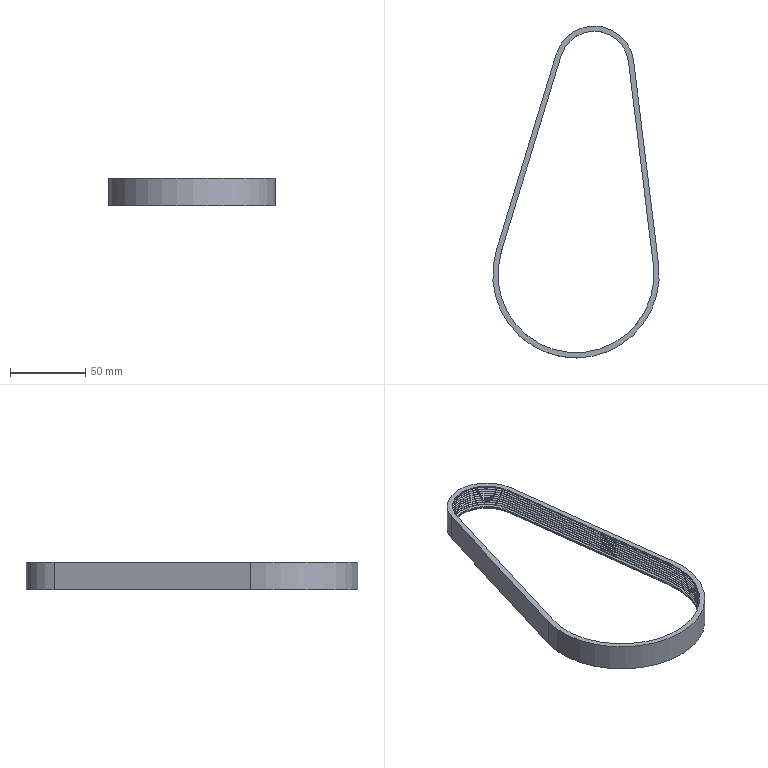Part | STEP file | DE200JS8 | 1 solid | 234 faces | box 111 x 221.3 x 18 mm | volume 22925 mm3 | cylinder 80 | plane 62 | torus 56 | cone 36 | commonest cylinder face diameters 0.4 x52 50 x9 108 x9 1 x4 46 x2 104 x2